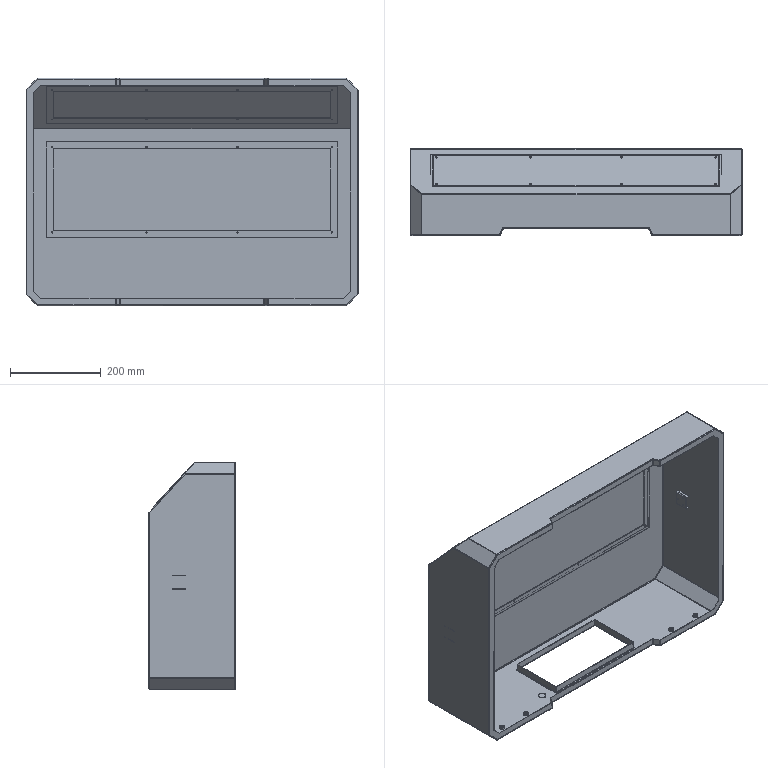Part | SolidWorks | 3 solids | 399 faces | box 730 x 190.8 x 500 mm | volume 1142428 mm3 | cylinder 218 | plane 121 | sphere 36 | spline 16 | torus 8 | commonest cylinder face diameters 4 x51 2.5 x44 2 x40 4.5 x32 1.6 x19 5 x8